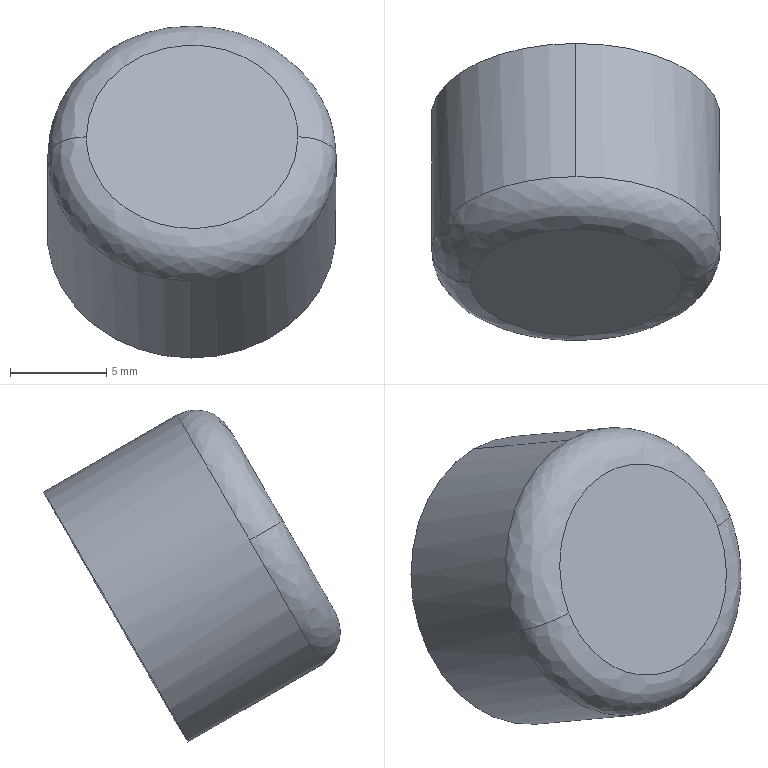Part | SolidWorks | features BaseBody 1 | 1 solid | 6 faces | box 15.03 x 15.428 x 17.258 mm | volume 1729 mm3 | spline 2 | cylinder 2 | plane 2 | commonest cylinder face diameters 15 x2
STEP:
#1=CARTESIAN_POINT('',(737.555,53.883,87.648));
#2=VERTEX_POINT('',#1);
#3=CARTESIAN_POINT('',(748.555,53.93,87.648));
#4=VERTEX_POINT('',#3);
#5=CARTESIAN_POINT('',(737.555,53.883,87.648));
#6=CARTESIAN_POINT('',(737.531,59.383,97.174));
#7=CARTESIAN_POINT('',(748.531,59.43,97.174));
#8=CARTESIAN_POINT('',(748.555,53.93,87.648));
#9=(BOUNDED_CURVE()B_SPLINE_CURVE(3,(#5,#6,#7,#8),.UNSPECIFIED.,.F.,.T.)B_SPLINE_CURVE_WITH_KNOTS((4,4),(0.,1.),.UNSPECIFIED.)CURVE()GEOMETRIC_REPRESENTATION_ITEM()RATIONAL_B_SPLINE_CURVE((1.,0.3333,0.3333,1.))REPRESENTATION_ITEM(''));
#10=EDGE_CURVE('',#2,#4,#9,.T.);
#11=ORIENTED_EDGE('',*,*,#10,.T.);
#12=CARTESIAN_POINT('',(750.547,55.671,86.648));
#13=VERTEX_POINT('',#12);
#14=CARTESIAN_POINT('',(748.547,55.662,86.648));
#15=DIRECTION('',(-0.002176,0.5,0.866));
#16=DIRECTION('',(1.,0.004352,-0.000000001));
#17=AXIS2_PLACEMENT_3D('',#14,#15,#16);
#18=CIRCLE('',#17,2.);
#19=EDGE_CURVE('',#4,#13,#18,.T.);
#20=ORIENTED_EDGE('',*,*,#19,.T.);
#21=CARTESIAN_POINT('',(743.047,59.389,93.143));
#22=VERTEX_POINT('',#21);
#23=CARTESIAN_POINT('',(743.047,55.639,86.648));
#24=DIRECTION('',(-0.003769,0.866,-0.5));
#25=DIRECTION('',(0.,0.5,0.866));
#26=AXIS2_PLACEMENT_3D('',#23,#24,#25);
#27=CIRCLE('',#26,7.5);
#28=EDGE_CURVE('',#22,#13,#27,.T.);
#29=ORIENTED_EDGE('',*,*,#28,.F.);
#30=CARTESIAN_POINT('',(735.547,55.606,86.648));
#31=VERTEX_POINT('',#30);
#32=CARTESIAN_POINT('',(743.047,55.639,86.648));
#33=DIRECTION('',(-0.003769,0.866,-0.5));
#34=DIRECTION('',(0.,0.5,0.866));
#35=AXIS2_PLACEMENT_3D('',#32,#33,#34);
#36=CIRCLE('',#35,7.5);
#37=EDGE_CURVE('',#31,#22,#36,.T.);
#38=ORIENTED_EDGE('',*,*,#37,.F.);
#39=CARTESIAN_POINT('',(737.547,55.615,86.648));
#40=DIRECTION('',(0.002176,-0.5,-0.866));
#41=DIRECTION('',(-1.,-0.004352,0.000000001));
#42=AXIS2_PLACEMENT_3D('',#39,#40,#41);
#43=CIRCLE('',#42,2.);
#44=EDGE_CURVE('',#2,#31,#43,.T.);
#45=ORIENTED_EDGE('',*,*,#44,.F.);
#46=EDGE_LOOP('',(#11,#20,#29,#38,#45));
#47=FACE_OUTER_BOUND('',#46,.T.);
#48=CARTESIAN_POINT('',(748.555,53.93,87.648));
#49=CARTESIAN_POINT('',(748.531,59.43,97.174));
#50=CARTESIAN_POINT('',(737.531,59.383,97.174));
#51=CARTESIAN_POINT('',(737.555,53.883,87.648));
#52=CARTESIAN_POINT('',(749.726,53.936,87.648));
#53=CARTESIAN_POINT('',(749.697,60.607,99.203));
#54=CARTESIAN_POINT('',(736.354,60.549,99.203));
#55=CARTESIAN_POINT('',(736.383,53.877,87.648));
#56=CARTESIAN_POINT('',(750.552,54.657,87.234));
#57=CARTESIAN_POINT('',(750.519,62.157,100.224));
#58=CARTESIAN_POINT('',(735.519,62.091,100.224));
#59=CARTESIAN_POINT('',(735.552,54.591,87.234));
#60=CARTESIAN_POINT('',(750.547,55.671,86.648));
#61=CARTESIAN_POINT('',(750.515,63.171,99.638));
#62=CARTESIAN_POINT('',(735.515,63.106,99.638));
#63=CARTESIAN_POINT('',(735.547,55.606,86.648));
#64=(BOUNDED_SURFACE()B_SPLINE_SURFACE(3,3,((#48,#49,#50,#51),(#52,#53,#54,#55),(#56,#57,#58,#59),(#60,#61,#62,#63)),.UNSPECIFIED.,.F.,.F.,.T.)B_SPLINE_SURFACE_WITH_KNOTS((4,4),(4,4),(0.,1.),(0.,1.),.UNSPECIFIED.)GEOMETRIC_REPRESENTATION_ITEM()RATIONAL_B_SPLINE_SURFACE(((1.,0.3333,0.3333,1.),(0.8047,0.2682,0.2682,0.8047),(0.8047,0.2682,0.2682,0.8047),(1.,0.3333,0.3333,1.)))REPRESENTATION_ITEM('')SURFACE());
#65=ADVANCED_FACE('',(#47),#64,.T.);
#66=ORIENTED_EDGE('',*,*,#28,.T.);
#67=CARTESIAN_POINT('',(743.047,51.889,80.153));
#68=VERTEX_POINT('',#67);
#69=CARTESIAN_POINT('',(743.047,55.639,86.648));
#70=DIRECTION('',(-0.003769,0.866,-0.5));
#71=DIRECTION('',(0.,0.5,0.866));
#72=AXIS2_PLACEMENT_3D('',#69,#70,#71);
#73=CIRCLE('',#72,7.5);
#74=EDGE_CURVE('',#13,#68,#73,.T.);
#75=ORIENTED_EDGE('',*,*,#74,.T.);
#76=CARTESIAN_POINT('',(743.017,58.817,76.153));
#77=VERTEX_POINT('',#76);
#78=CARTESIAN_POINT('',(743.017,58.817,76.153));
#79=DIRECTION('',(-0.003769,0.866,-0.5));
#80=VECTOR('',#79,1000.);
#81=LINE('',#78,#80);
#82=EDGE_CURVE('',#68,#77,#81,.T.);
#83=ORIENTED_EDGE('',*,*,#82,.T.);
#84=CARTESIAN_POINT('',(743.017,66.317,89.143));
#85=VERTEX_POINT('',#84);
#86=CARTESIAN_POINT('',(743.017,62.567,82.648));
#87=DIRECTION('',(0.003769,-0.866,0.5));
#88=DIRECTION('',(0.,0.5,0.866));
#89=AXIS2_PLACEMENT_3D('',#86,#87,#88);
#90=CIRCLE('',#89,7.5);
#91=EDGE_CURVE('',#77,#85,#90,.T.);
#92=ORIENTED_EDGE('',*,*,#91,.T.);
#93=CARTESIAN_POINT('',(743.017,66.317,89.143));
#94=DIRECTION('',(-0.003769,0.866,-0.5));
#95=VECTOR('',#94,1000.);
#96=LINE('',#93,#95);
#97=EDGE_CURVE('',#22,#85,#96,.T.);
#98=ORIENTED_EDGE('',*,*,#97,.F.);
#99=EDGE_LOOP('',(#66,#75,#83,#92,#98));
#100=FACE_OUTER_BOUND('',#99,.T.);
#101=CARTESIAN_POINT('',(743.017,62.567,82.648));
#102=DIRECTION('',(-0.003769,0.866,-0.5));
#103=DIRECTION('',(0.,0.5,0.866));
#104=AXIS2_PLACEMENT_3D('',#101,#102,#103);
#105=CYLINDRICAL_SURFACE('',#104,7.5);
#106=ADVANCED_FACE('',(#100),#105,.T.);
#107=ORIENTED_EDGE('',*,*,#82,.F.);
#108=CARTESIAN_POINT('',(743.047,55.639,86.648));
#109=DIRECTION('',(-0.003769,0.866,-0.5));
#110=DIRECTION('',(0.,0.5,0.866));
#111=AXIS2_PLACEMENT_3D('',#108,#109,#110);
#112=CIRCLE('',#111,7.5);
#113=EDGE_CURVE('',#68,#31,#112,.T.);
#114=ORIENTED_EDGE('',*,*,#113,.T.);
#115=ORIENTED_EDGE('',*,*,#37,.T.);
#116=ORIENTED_EDGE('',*,*,#97,.T.);
#117=CARTESIAN_POINT('',(743.017,62.567,82.648));
#118=DIRECTION('',(0.003769,-0.866,0.5));
#119=DIRECTION('',(0.,0.5,0.866));
#120=AXIS2_PLACEMENT_3D('',#117,#118,#119);
#121=CIRCLE('',#120,7.5);
#122=EDGE_CURVE('',#85,#77,#121,.T.);
#123=ORIENTED_EDGE('',*,*,#122,.T.);
#124=EDGE_LOOP('',(#107,#114,#115,#116,#123));
#125=FACE_OUTER_BOUND('',#124,.T.);
#126=CARTESIAN_POINT('',(743.017,62.567,82.648));
#127=DIRECTION('',(-0.003769,0.866,-0.5));
#128=DIRECTION('',(0.,0.5,0.866));
#129=AXIS2_PLACEMENT_3D('',#126,#127,#128);
#130=CYLINDRICAL_SURFACE('',#129,7.5);
#131=ADVANCED_FACE('',(#125),#130,.T.);
#132=ORIENTED_EDGE('',*,*,#122,.F.);
#133=ORIENTED_EDGE('',*,*,#91,.F.);
#134=EDGE_LOOP('',(#132,#133));
#135=FACE_OUTER_BOUND('',#134,.T.);
#136=CARTESIAN_POINT('',(743.017,62.567,82.648));
#137=DIRECTION('',(0.003769,-0.866,0.5));
#138=DIRECTION('',(0.,-0.5,-0.866));
#139=AXIS2_PLACEMENT_3D('',#136,#137,#138);
#140=PLANE('',#139);
#141=ADVANCED_FACE('',(#135),#140,.F.);
#142=ORIENTED_EDGE('',*,*,#19,.F.);
#143=CARTESIAN_POINT('',(748.555,53.93,87.648));
#144=CARTESIAN_POINT('',(748.579,48.431,78.122));
#145=CARTESIAN_POINT('',(737.579,48.383,78.122));
#146=CARTESIAN_POINT('',(737.555,53.883,87.648));
#147=(BOUNDED_CURVE()B_SPLINE_CURVE(3,(#143,#144,#145,#146),.UNSPECIFIED.,.F.,.T.)B_SPLINE_CURVE_WITH_KNOTS((4,4),(0.,1.),.UNSPECIFIED.)CURVE()GEOMETRIC_REPRESENTATION_ITEM()RATIONAL_B_SPLINE_CURVE((1.,0.3333,0.3333,1.))REPRESENTATION_ITEM(''));
#148=EDGE_CURVE('',#4,#2,#147,.T.);
#149=ORIENTED_EDGE('',*,*,#148,.T.);
#150=ORIENTED_EDGE('',*,*,#44,.T.);
#151=ORIENTED_EDGE('',*,*,#113,.F.);
#152=ORIENTED_EDGE('',*,*,#74,.F.);
#153=EDGE_LOOP('',(#142,#149,#150,#151,#152));
#154=FACE_OUTER_BOUND('',#153,.T.);
#155=CARTESIAN_POINT('',(737.555,53.883,87.648));
#156=CARTESIAN_POINT('',(737.579,48.383,78.122));
#157=CARTESIAN_POINT('',(748.579,48.431,78.122));
#158=CARTESIAN_POINT('',(748.555,53.93,87.648));
#159=CARTESIAN_POINT('',(736.383,53.877,87.648));
#160=CARTESIAN_POINT('',(736.412,47.206,76.092));
#161=CARTESIAN_POINT('',(749.755,47.264,76.092));
#162=CARTESIAN_POINT('',(749.726,53.936,87.648));
#163=CARTESIAN_POINT('',(735.552,54.591,87.234));
#164=CARTESIAN_POINT('',(735.584,47.091,74.243));
#165=CARTESIAN_POINT('',(750.584,47.157,74.243));
#166=CARTESIAN_POINT('',(750.552,54.657,87.234));
#167=CARTESIAN_POINT('',(735.547,55.606,86.648));
#168=CARTESIAN_POINT('',(735.58,48.106,73.657));
#169=CARTESIAN_POINT('',(750.58,48.171,73.657));
#170=CARTESIAN_POINT('',(750.547,55.671,86.648));
#171=(BOUNDED_SURFACE()B_SPLINE_SURFACE(3,3,((#155,#156,#157,#158),(#159,#160,#161,#162),(#163,#164,#165,#166),(#167,#168,#169,#170)),.UNSPECIFIED.,.F.,.F.,.F.)B_SPLINE_SURFACE_WITH_KNOTS((4,4),(4,4),(0.,1.),(0.,1.),.UNSPECIFIED.)GEOMETRIC_REPRESENTATION_ITEM()RATIONAL_B_SPLINE_SURFACE(((1.,0.3333,0.3333,1.),(0.8047,0.2682,0.2682,0.8047),(0.8047,0.2682,0.2682,0.8047),(1.,0.3333,0.3333,1.)))REPRESENTATION_ITEM('')SURFACE());
#172=ADVANCED_FACE('',(#154),#171,.T.);
#173=ORIENTED_EDGE('',*,*,#148,.F.);
#174=ORIENTED_EDGE('',*,*,#10,.F.);
#175=EDGE_LOOP('',(#173,#174));
#176=FACE_OUTER_BOUND('',#175,.T.);
#177=CARTESIAN_POINT('',(743.055,53.907,87.648));
#178=DIRECTION('',(0.003769,-0.866,0.5));
#179=DIRECTION('',(0.,-0.5,-0.866));
#180=AXIS2_PLACEMENT_3D('',#177,#178,#179);
#181=PLANE('',#180);
#182=ADVANCED_FACE('',(#176),#181,.T.);
#183=CLOSED_SHELL('',(#65,#106,#131,#141,#172,#182));
#184=MANIFOLD_SOLID_BREP('',#183);
#185=CARTESIAN_POINT('',(0.,0.,0.));
#186=DIRECTION('',(0.,0.,1.));
#187=DIRECTION('',(1.,0.,0.));
#188=AXIS2_PLACEMENT_3D('',#185,#186,#187);
#189=(LENGTH_UNIT()NAMED_UNIT(*)SI_UNIT(.MILLI.,.METRE.));
#190=UNCERTAINTY_MEASURE_WITH_UNIT(LENGTH_MEASURE(0.00001),#189,'','');
#191=(NAMED_UNIT(*)PLANE_ANGLE_UNIT()SI_UNIT($,.RADIAN.));
#192=(NAMED_UNIT(*)SI_UNIT($,.STERADIAN.)SOLID_ANGLE_UNIT());
#193=(GEOMETRIC_REPRESENTATION_CONTEXT(3)GLOBAL_UNCERTAINTY_ASSIGNED_CONTEXT((#190))GLOBAL_UNIT_ASSIGNED_CONTEXT((#189,#191,#192))REPRESENTATION_CONTEXT('',''));
#194=ADVANCED_BREP_SHAPE_REPRESENTATION('',(#184,#188),#193);